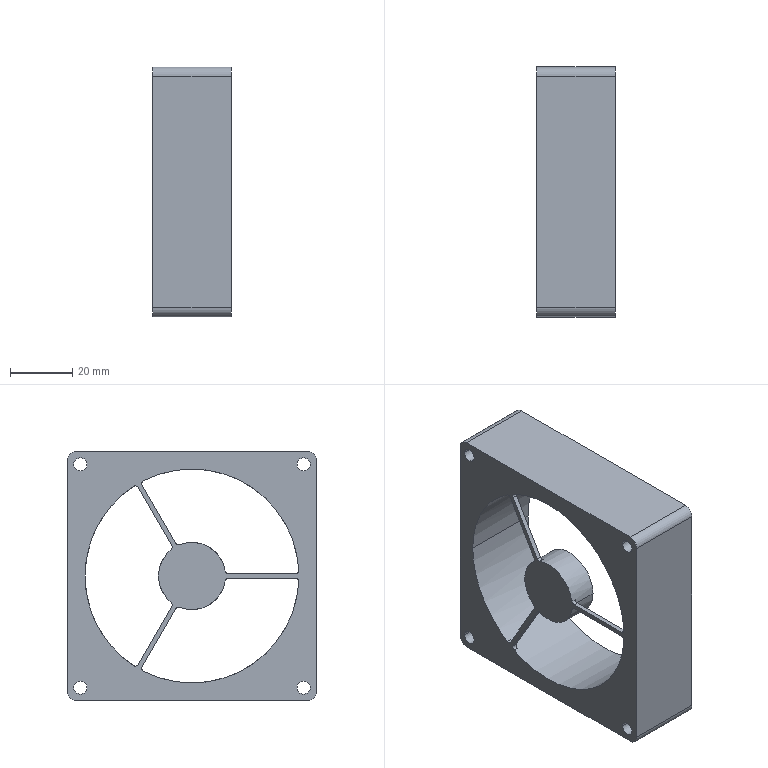Part | STEP file | Axial Fan RDH8025B2_24V DC_3000RPM_ECO | 1 solid | 44 faces | box 25 x 80 x 80 mm | volume 69901 mm3 | cylinder 28 | plane 16 | commonest cylinder face diameters 2 x12 4.2 x8 6 x4 21.5 x2 68.5 x2